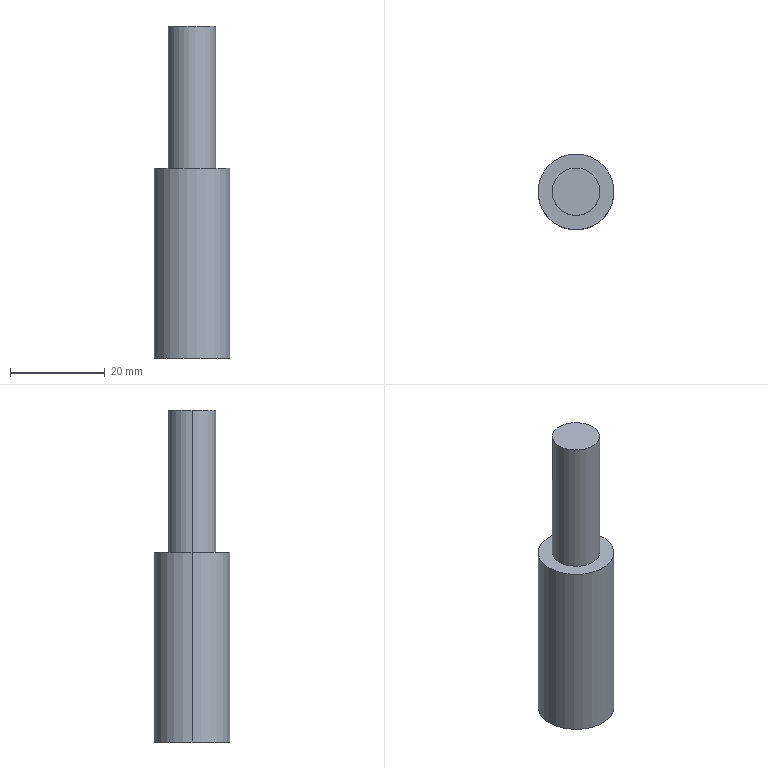Part | SolidWorks | features Extrusion 1, ICE 1 | 1 solid | 7 faces | box 16 x 16 x 70 mm | volume 10399 mm3 | cylinder 4 | plane 3 | commonest cylinder face diameters 10 x2 16 x2
STEP:
#1=CARTESIAN_POINT('',(5.,0.,70.));
#2=VERTEX_POINT('',#1);
#3=CARTESIAN_POINT('',(-5.,0.,70.));
#4=VERTEX_POINT('',#3);
#5=CARTESIAN_POINT('',(0.,0.,70.));
#6=DIRECTION('',(0.,0.,1.));
#7=DIRECTION('',(1.,0.,0.));
#8=AXIS2_PLACEMENT_3D('',#5,#6,#7);
#9=CIRCLE('',#8,5.);
#10=EDGE_CURVE('',#2,#4,#9,.T.);
#11=ORIENTED_EDGE('',*,*,#10,.F.);
#12=CARTESIAN_POINT('',(5.,0.,40.));
#13=VERTEX_POINT('',#12);
#14=CARTESIAN_POINT('',(5.,0.,70.));
#15=DIRECTION('',(0.,0.,-1.));
#16=VECTOR('',#15,1000.);
#17=LINE('',#14,#16);
#18=EDGE_CURVE('',#2,#13,#17,.T.);
#19=ORIENTED_EDGE('',*,*,#18,.T.);
#20=CARTESIAN_POINT('',(-5.,0.,40.));
#21=VERTEX_POINT('',#20);
#22=CARTESIAN_POINT('',(0.,0.,40.));
#23=DIRECTION('',(0.,0.,1.));
#24=DIRECTION('',(1.,0.,0.));
#25=AXIS2_PLACEMENT_3D('',#22,#23,#24);
#26=CIRCLE('',#25,5.);
#27=EDGE_CURVE('',#13,#21,#26,.T.);
#28=ORIENTED_EDGE('',*,*,#27,.T.);
#29=CARTESIAN_POINT('',(-5.,0.,70.));
#30=DIRECTION('',(0.,0.,-1.));
#31=VECTOR('',#30,1000.);
#32=LINE('',#29,#31);
#33=EDGE_CURVE('',#4,#21,#32,.T.);
#34=ORIENTED_EDGE('',*,*,#33,.F.);
#35=EDGE_LOOP('',(#11,#19,#28,#34));
#36=FACE_OUTER_BOUND('',#35,.T.);
#37=CARTESIAN_POINT('',(0.,0.,70.));
#38=DIRECTION('',(0.,0.,-1.));
#39=DIRECTION('',(-1.,0.,0.));
#40=AXIS2_PLACEMENT_3D('',#37,#38,#39);
#41=CYLINDRICAL_SURFACE('',#40,5.);
#42=ADVANCED_FACE('',(#36),#41,.T.);
#43=CARTESIAN_POINT('',(8.,0.,40.));
#44=VERTEX_POINT('',#43);
#45=CARTESIAN_POINT('',(-8.,0.,40.));
#46=VERTEX_POINT('',#45);
#47=CARTESIAN_POINT('',(0.,0.,40.));
#48=DIRECTION('',(0.,0.,1.));
#49=DIRECTION('',(1.,0.,0.));
#50=AXIS2_PLACEMENT_3D('',#47,#48,#49);
#51=CIRCLE('',#50,8.);
#52=EDGE_CURVE('',#44,#46,#51,.T.);
#53=ORIENTED_EDGE('',*,*,#52,.F.);
#54=CARTESIAN_POINT('',(8.,0.,0.));
#55=VERTEX_POINT('',#54);
#56=CARTESIAN_POINT('',(8.,0.,40.));
#57=DIRECTION('',(0.,0.,-1.));
#58=VECTOR('',#57,1000.);
#59=LINE('',#56,#58);
#60=EDGE_CURVE('',#44,#55,#59,.T.);
#61=ORIENTED_EDGE('',*,*,#60,.T.);
#62=CARTESIAN_POINT('',(-8.,0.,0.));
#63=VERTEX_POINT('',#62);
#64=CARTESIAN_POINT('',(0.,0.,0.));
#65=DIRECTION('',(0.,0.,1.));
#66=DIRECTION('',(1.,0.,0.));
#67=AXIS2_PLACEMENT_3D('',#64,#65,#66);
#68=CIRCLE('',#67,8.);
#69=EDGE_CURVE('',#55,#63,#68,.T.);
#70=ORIENTED_EDGE('',*,*,#69,.T.);
#71=CARTESIAN_POINT('',(-8.,0.,40.));
#72=DIRECTION('',(0.,0.,-1.));
#73=VECTOR('',#72,1000.);
#74=LINE('',#71,#73);
#75=EDGE_CURVE('',#46,#63,#74,.T.);
#76=ORIENTED_EDGE('',*,*,#75,.F.);
#77=EDGE_LOOP('',(#53,#61,#70,#76));
#78=FACE_OUTER_BOUND('',#77,.T.);
#79=CARTESIAN_POINT('',(0.,0.,40.));
#80=DIRECTION('',(0.,0.,-1.));
#81=DIRECTION('',(-1.,0.,0.));
#82=AXIS2_PLACEMENT_3D('',#79,#80,#81);
#83=CYLINDRICAL_SURFACE('',#82,8.);
#84=ADVANCED_FACE('',(#78),#83,.T.);
#85=CARTESIAN_POINT('',(0.,0.,40.));
#86=DIRECTION('',(0.,0.,1.));
#87=DIRECTION('',(1.,0.,0.));
#88=AXIS2_PLACEMENT_3D('',#85,#86,#87);
#89=CIRCLE('',#88,8.);
#90=EDGE_CURVE('',#46,#44,#89,.T.);
#91=ORIENTED_EDGE('',*,*,#90,.T.);
#92=ORIENTED_EDGE('',*,*,#52,.T.);
#93=EDGE_LOOP('',(#91,#92));
#94=FACE_OUTER_BOUND('',#93,.T.);
#95=CARTESIAN_POINT('',(0.,0.,40.));
#96=DIRECTION('',(0.,0.,1.));
#97=DIRECTION('',(1.,0.,0.));
#98=AXIS2_PLACEMENT_3D('',#95,#96,#97);
#99=CIRCLE('',#98,5.);
#100=EDGE_CURVE('',#21,#13,#99,.T.);
#101=ORIENTED_EDGE('',*,*,#100,.F.);
#102=ORIENTED_EDGE('',*,*,#27,.F.);
#103=EDGE_LOOP('',(#101,#102));
#104=FACE_BOUND('',#103,.T.);
#105=CARTESIAN_POINT('',(0.,0.,40.));
#106=DIRECTION('',(0.,0.,1.));
#107=DIRECTION('',(1.,0.,0.));
#108=AXIS2_PLACEMENT_3D('',#105,#106,#107);
#109=PLANE('',#108);
#110=ADVANCED_FACE('',(#94,#104),#109,.T.);
#111=ORIENTED_EDGE('',*,*,#60,.F.);
#112=ORIENTED_EDGE('',*,*,#90,.F.);
#113=ORIENTED_EDGE('',*,*,#75,.T.);
#114=CARTESIAN_POINT('',(0.,0.,0.));
#115=DIRECTION('',(0.,0.,1.));
#116=DIRECTION('',(1.,0.,0.));
#117=AXIS2_PLACEMENT_3D('',#114,#115,#116);
#118=CIRCLE('',#117,8.);
#119=EDGE_CURVE('',#63,#55,#118,.T.);
#120=ORIENTED_EDGE('',*,*,#119,.T.);
#121=EDGE_LOOP('',(#111,#112,#113,#120));
#122=FACE_OUTER_BOUND('',#121,.T.);
#123=CARTESIAN_POINT('',(0.,0.,40.));
#124=DIRECTION('',(0.,0.,-1.));
#125=DIRECTION('',(-1.,0.,0.));
#126=AXIS2_PLACEMENT_3D('',#123,#124,#125);
#127=CYLINDRICAL_SURFACE('',#126,8.);
#128=ADVANCED_FACE('',(#122),#127,.T.);
#129=ORIENTED_EDGE('',*,*,#119,.F.);
#130=ORIENTED_EDGE('',*,*,#69,.F.);
#131=EDGE_LOOP('',(#129,#130));
#132=FACE_OUTER_BOUND('',#131,.T.);
#133=CARTESIAN_POINT('',(0.,0.,0.));
#134=DIRECTION('',(0.,0.,1.));
#135=DIRECTION('',(1.,0.,0.));
#136=AXIS2_PLACEMENT_3D('',#133,#134,#135);
#137=PLANE('',#136);
#138=ADVANCED_FACE('',(#132),#137,.F.);
#139=ORIENTED_EDGE('',*,*,#18,.F.);
#140=CARTESIAN_POINT('',(0.,0.,70.));
#141=DIRECTION('',(0.,0.,1.));
#142=DIRECTION('',(1.,0.,0.));
#143=AXIS2_PLACEMENT_3D('',#140,#141,#142);
#144=CIRCLE('',#143,5.);
#145=EDGE_CURVE('',#4,#2,#144,.T.);
#146=ORIENTED_EDGE('',*,*,#145,.F.);
#147=ORIENTED_EDGE('',*,*,#33,.T.);
#148=ORIENTED_EDGE('',*,*,#100,.T.);
#149=EDGE_LOOP('',(#139,#146,#147,#148));
#150=FACE_OUTER_BOUND('',#149,.T.);
#151=CARTESIAN_POINT('',(0.,0.,70.));
#152=DIRECTION('',(0.,0.,-1.));
#153=DIRECTION('',(-1.,0.,0.));
#154=AXIS2_PLACEMENT_3D('',#151,#152,#153);
#155=CYLINDRICAL_SURFACE('',#154,5.);
#156=ADVANCED_FACE('',(#150),#155,.T.);
#157=ORIENTED_EDGE('',*,*,#145,.T.);
#158=ORIENTED_EDGE('',*,*,#10,.T.);
#159=EDGE_LOOP('',(#157,#158));
#160=FACE_OUTER_BOUND('',#159,.T.);
#161=CARTESIAN_POINT('',(0.,0.,70.));
#162=DIRECTION('',(0.,0.,1.));
#163=DIRECTION('',(1.,0.,0.));
#164=AXIS2_PLACEMENT_3D('',#161,#162,#163);
#165=PLANE('',#164);
#166=ADVANCED_FACE('',(#160),#165,.T.);
#167=CLOSED_SHELL('',(#42,#84,#110,#128,#138,#156,#166));
#168=MANIFOLD_SOLID_BREP('',#167);
#169=CARTESIAN_POINT('',(0.,0.,0.));
#170=DIRECTION('',(0.,0.,1.));
#171=DIRECTION('',(1.,0.,0.));
#172=AXIS2_PLACEMENT_3D('',#169,#170,#171);
#173=(LENGTH_UNIT()NAMED_UNIT(*)SI_UNIT(.MILLI.,.METRE.));
#174=UNCERTAINTY_MEASURE_WITH_UNIT(LENGTH_MEASURE(0.00001),#173,'','');
#175=(NAMED_UNIT(*)PLANE_ANGLE_UNIT()SI_UNIT($,.RADIAN.));
#176=(NAMED_UNIT(*)SI_UNIT($,.STERADIAN.)SOLID_ANGLE_UNIT());
#177=(GEOMETRIC_REPRESENTATION_CONTEXT(3)GLOBAL_UNCERTAINTY_ASSIGNED_CONTEXT((#174))GLOBAL_UNIT_ASSIGNED_CONTEXT((#173,#175,#176))REPRESENTATION_CONTEXT('',''));
#178=ADVANCED_BREP_SHAPE_REPRESENTATION('',(#168,#172),#177);